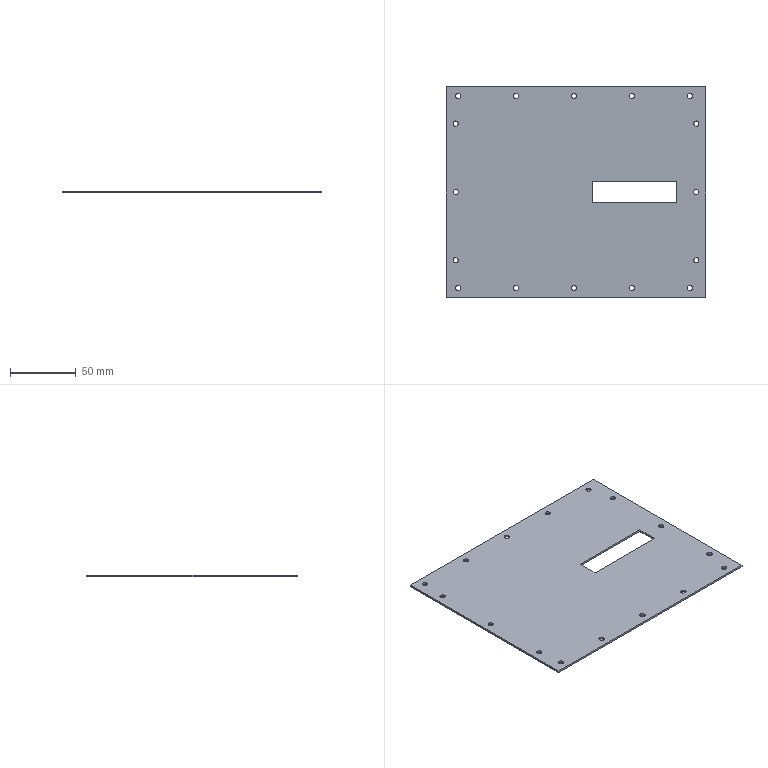Part | STEP file | 1-43.12 | 1 solid | 26 faces | box 197 x 160 x 1.5 mm | volume 45442 mm3 | cylinder 16 | plane 10 | commonest cylinder face diameters 4 x16